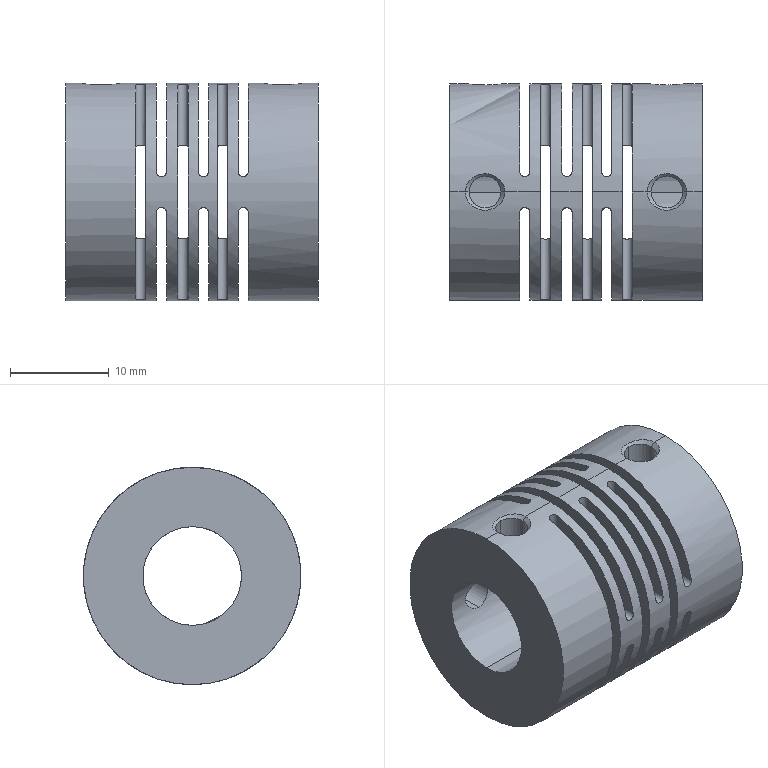Part | SolidWorks | features BaseBody 1 | 1 solid | 76 faces | box 25.6 x 22 x 22 mm | volume 5890 mm3 | cylinder 42 | plane 26 | cone 8 | commonest cylinder face diameters 1.04 x30 3.242 x8 10 x2 22 x2